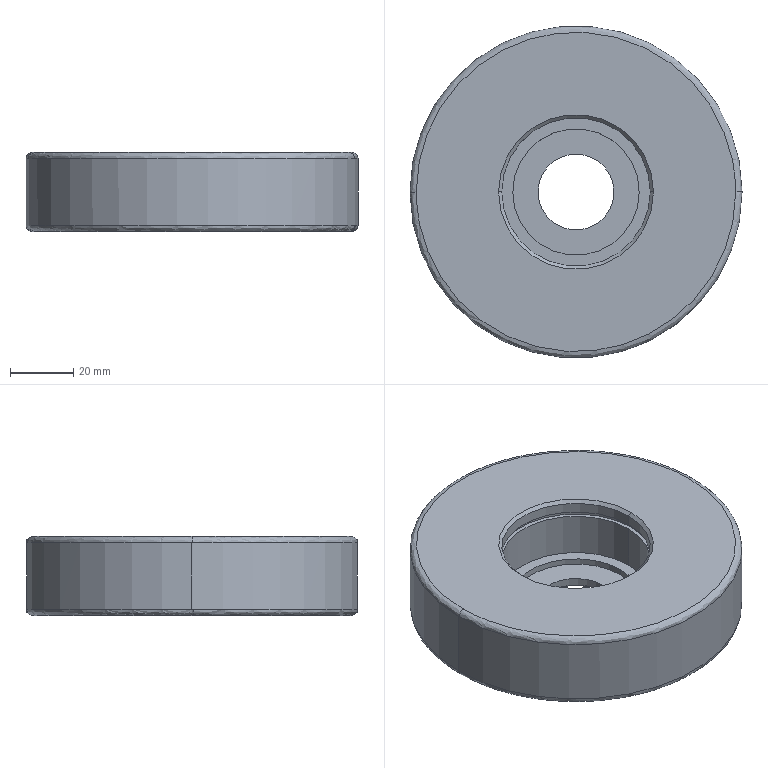Part | SolidWorks | features BaseBody 1 | 1 solid | 26 faces | box 105 x 105 x 25 mm | volume 176949 mm3 | cylinder 12 | plane 6 | spline 4 | cone 4 | commonest cylinder face diameters 47 x4 24 x2 40 x2 49.5 x2 105 x2
STEP:
#1=CARTESIAN_POINT('',(-52.5,0.,-23.));
#2=VERTEX_POINT('',#1);
#3=CARTESIAN_POINT('',(52.499,0.3289,-23.));
#4=VERTEX_POINT('',#3);
#5=CARTESIAN_POINT('',(0.,0.,-23.));
#6=DIRECTION('',(0.,0.,-1.));
#7=DIRECTION('',(-1.,-0.006265,0.));
#8=AXIS2_PLACEMENT_3D('',#5,#6,#7);
#9=CIRCLE('',#8,52.5);
#10=EDGE_CURVE('',#2,#4,#9,.T.);
#11=ORIENTED_EDGE('',*,*,#10,.T.);
#12=CARTESIAN_POINT('',(50.499,0.3164,-25.));
#13=VERTEX_POINT('',#12);
#14=CARTESIAN_POINT('',(50.499,0.3164,-23.));
#15=DIRECTION('',(-0.006265,1.,0.));
#16=DIRECTION('',(1.,0.006265,0.));
#17=AXIS2_PLACEMENT_3D('',#14,#15,#16);
#18=CIRCLE('',#17,2.);
#19=EDGE_CURVE('',#4,#13,#18,.T.);
#20=ORIENTED_EDGE('',*,*,#19,.T.);
#21=CARTESIAN_POINT('',(-50.5,0.,-25.));
#22=VERTEX_POINT('',#21);
#23=CARTESIAN_POINT('',(50.499,0.3164,-25.));
#24=CARTESIAN_POINT('',(49.87,100.685,-25.));
#25=CARTESIAN_POINT('',(-50.5,100.371,-25.));
#26=CARTESIAN_POINT('',(-50.5,0.,-25.));
#27=(BOUNDED_CURVE()B_SPLINE_CURVE(3,(#23,#24,#25,#26),.UNSPECIFIED.,.F.,.F.)B_SPLINE_CURVE_WITH_KNOTS((4,4),(0.001994,1.),.UNSPECIFIED.)CURVE()GEOMETRIC_REPRESENTATION_ITEM()RATIONAL_B_SPLINE_CURVE((1.,0.3354,0.3354,1.))REPRESENTATION_ITEM(''));
#28=EDGE_CURVE('',#13,#22,#27,.T.);
#29=ORIENTED_EDGE('',*,*,#28,.T.);
#30=CARTESIAN_POINT('',(-50.499,-0.3164,-25.));
#31=VERTEX_POINT('',#30);
#32=CARTESIAN_POINT('',(-50.5,0.,-25.));
#33=CARTESIAN_POINT('',(-50.5,-0.1055,-25.));
#34=CARTESIAN_POINT('',(-50.5,-0.2109,-25.));
#35=CARTESIAN_POINT('',(-50.499,-0.3164,-25.));
#36=(BOUNDED_CURVE()B_SPLINE_CURVE(3,(#32,#33,#34,#35),.UNSPECIFIED.,.F.,.F.)B_SPLINE_CURVE_WITH_KNOTS((4,4),(0.,0.001994),.UNSPECIFIED.)CURVE()GEOMETRIC_REPRESENTATION_ITEM()RATIONAL_B_SPLINE_CURVE((1.,1.,1.,1.))REPRESENTATION_ITEM(''));
#37=EDGE_CURVE('',#22,#31,#36,.T.);
#38=ORIENTED_EDGE('',*,*,#37,.T.);
#39=CARTESIAN_POINT('',(-52.499,-0.3289,-23.));
#40=VERTEX_POINT('',#39);
#41=CARTESIAN_POINT('',(-50.499,-0.3164,-23.));
#42=DIRECTION('',(0.006265,-1.,0.));
#43=DIRECTION('',(-1.,-0.006265,0.));
#44=AXIS2_PLACEMENT_3D('',#41,#42,#43);
#45=CIRCLE('',#44,2.);
#46=EDGE_CURVE('',#40,#31,#45,.T.);
#47=ORIENTED_EDGE('',*,*,#46,.F.);
#48=CARTESIAN_POINT('',(0.,0.,-23.));
#49=DIRECTION('',(0.,0.,-1.));
#50=DIRECTION('',(-1.,-0.006265,0.));
#51=AXIS2_PLACEMENT_3D('',#48,#49,#50);
#52=CIRCLE('',#51,52.5);
#53=EDGE_CURVE('',#40,#2,#52,.T.);
#54=ORIENTED_EDGE('',*,*,#53,.T.);
#55=EDGE_LOOP('',(#11,#20,#29,#38,#47,#54));
#56=FACE_OUTER_BOUND('',#55,.T.);
#57=CARTESIAN_POINT('',(52.499,0.3289,-23.));
#58=CARTESIAN_POINT('',(51.841,105.327,-23.));
#59=CARTESIAN_POINT('',(-53.157,104.669,-23.));
#60=CARTESIAN_POINT('',(-52.499,-0.3289,-23.));
#61=CARTESIAN_POINT('',(52.499,0.3289,-24.172));
#62=CARTESIAN_POINT('',(51.841,105.327,-24.172));
#63=CARTESIAN_POINT('',(-53.157,104.669,-24.172));
#64=CARTESIAN_POINT('',(-52.499,-0.3289,-24.172));
#65=CARTESIAN_POINT('',(51.671,0.3237,-25.));
#66=CARTESIAN_POINT('',(51.023,103.665,-25.));
#67=CARTESIAN_POINT('',(-52.318,103.017,-25.));
#68=CARTESIAN_POINT('',(-51.671,-0.3237,-25.));
#69=CARTESIAN_POINT('',(50.499,0.3164,-25.));
#70=CARTESIAN_POINT('',(49.866,101.314,-25.));
#71=CARTESIAN_POINT('',(-51.132,100.682,-25.));
#72=CARTESIAN_POINT('',(-50.499,-0.3164,-25.));
#73=(BOUNDED_SURFACE()B_SPLINE_SURFACE(3,3,((#57,#58,#59,#60),(#61,#62,#63,#64),(#65,#66,#67,#68),(#69,#70,#71,#72)),.UNSPECIFIED.,.F.,.F.,.T.)B_SPLINE_SURFACE_WITH_KNOTS((4,4),(4,4),(0.,1.),(0.,1.),.UNSPECIFIED.)GEOMETRIC_REPRESENTATION_ITEM()RATIONAL_B_SPLINE_SURFACE(((1.,0.3333,0.3333,1.),(0.8047,0.2682,0.2682,0.8047),(0.8047,0.2682,0.2682,0.8047),(1.,0.3333,0.3333,1.)))REPRESENTATION_ITEM('')SURFACE());
#74=ADVANCED_FACE('',(#56),#73,.T.);
#75=CARTESIAN_POINT('',(-50.5,0.,0.));
#76=VERTEX_POINT('',#75);
#77=CARTESIAN_POINT('',(50.5,0.2141,0.));
#78=VERTEX_POINT('',#77);
#79=CARTESIAN_POINT('',(-50.5,0.,0.));
#80=CARTESIAN_POINT('',(-50.5,100.573,0.));
#81=CARTESIAN_POINT('',(50.073,100.787,0.));
#82=CARTESIAN_POINT('',(50.5,0.2141,0.));
#83=(BOUNDED_CURVE()B_SPLINE_CURVE(3,(#79,#80,#81,#82),.UNSPECIFIED.,.F.,.F.)B_SPLINE_CURVE_WITH_KNOTS((4,4),(0.,0.9987),.UNSPECIFIED.)CURVE()GEOMETRIC_REPRESENTATION_ITEM()RATIONAL_B_SPLINE_CURVE((1.,0.3347,0.3347,1.))REPRESENTATION_ITEM(''));
#84=EDGE_CURVE('',#76,#78,#83,.T.);
#85=ORIENTED_EDGE('',*,*,#84,.T.);
#86=CARTESIAN_POINT('',(52.5,0.2226,-2.));
#87=VERTEX_POINT('',#86);
#88=CARTESIAN_POINT('',(50.5,0.2141,-2.));
#89=DIRECTION('',(-0.004241,1.,0.));
#90=DIRECTION('',(1.,0.004241,0.));
#91=AXIS2_PLACEMENT_3D('',#88,#89,#90);
#92=CIRCLE('',#91,2.);
#93=EDGE_CURVE('',#78,#87,#92,.T.);
#94=ORIENTED_EDGE('',*,*,#93,.T.);
#95=CARTESIAN_POINT('',(-52.5,0.,-2.));
#96=VERTEX_POINT('',#95);
#97=CARTESIAN_POINT('',(0.,0.,-2.));
#98=DIRECTION('',(0.,0.,-1.));
#99=DIRECTION('',(1.,0.,0.));
#100=AXIS2_PLACEMENT_3D('',#97,#98,#99);
#101=CIRCLE('',#100,52.5);
#102=EDGE_CURVE('',#96,#87,#101,.T.);
#103=ORIENTED_EDGE('',*,*,#102,.F.);
#104=CARTESIAN_POINT('',(-52.5,-0.2226,-2.));
#105=VERTEX_POINT('',#104);
#106=CARTESIAN_POINT('',(0.,0.,-2.));
#107=DIRECTION('',(0.,0.,-1.));
#108=DIRECTION('',(1.,0.,0.));
#109=AXIS2_PLACEMENT_3D('',#106,#107,#108);
#110=CIRCLE('',#109,52.5);
#111=EDGE_CURVE('',#105,#96,#110,.T.);
#112=ORIENTED_EDGE('',*,*,#111,.F.);
#113=CARTESIAN_POINT('',(-50.5,-0.2141,0.));
#114=VERTEX_POINT('',#113);
#115=CARTESIAN_POINT('',(-50.5,-0.2141,-2.));
#116=DIRECTION('',(0.004241,-1.,0.));
#117=DIRECTION('',(-1.,-0.004241,0.));
#118=AXIS2_PLACEMENT_3D('',#115,#116,#117);
#119=CIRCLE('',#118,2.);
#120=EDGE_CURVE('',#114,#105,#119,.T.);
#121=ORIENTED_EDGE('',*,*,#120,.F.);
#122=CARTESIAN_POINT('',(-50.5,-0.2141,0.));
#123=CARTESIAN_POINT('',(-50.5,-0.1428,0.));
#124=CARTESIAN_POINT('',(-50.5,-0.07138,0.));
#125=CARTESIAN_POINT('',(-50.5,0.,0.));
#126=(BOUNDED_CURVE()B_SPLINE_CURVE(3,(#122,#123,#124,#125),.UNSPECIFIED.,.F.,.F.)B_SPLINE_CURVE_WITH_KNOTS((4,4),(0.9987,1.),.UNSPECIFIED.)CURVE()GEOMETRIC_REPRESENTATION_ITEM()RATIONAL_B_SPLINE_CURVE((1.,1.,1.,1.))REPRESENTATION_ITEM(''));
#127=EDGE_CURVE('',#114,#76,#126,.T.);
#128=ORIENTED_EDGE('',*,*,#127,.T.);
#129=EDGE_LOOP('',(#85,#94,#103,#112,#121,#128));
#130=FACE_OUTER_BOUND('',#129,.T.);
#131=CARTESIAN_POINT('',(50.5,0.2141,0.));
#132=CARTESIAN_POINT('',(50.071,101.213,0.));
#133=CARTESIAN_POINT('',(-50.928,100.785,0.));
#134=CARTESIAN_POINT('',(-50.5,-0.2141,0.));
#135=CARTESIAN_POINT('',(51.671,0.2191,0.));
#136=CARTESIAN_POINT('',(51.233,103.561,0.));
#137=CARTESIAN_POINT('',(-52.109,103.123,0.));
#138=CARTESIAN_POINT('',(-51.671,-0.2191,0.));
#139=CARTESIAN_POINT('',(52.5,0.2226,-0.8284));
#140=CARTESIAN_POINT('',(52.054,105.222,-0.8284));
#141=CARTESIAN_POINT('',(-52.945,104.776,-0.8284));
#142=CARTESIAN_POINT('',(-52.5,-0.2226,-0.8284));
#143=CARTESIAN_POINT('',(52.5,0.2226,-2.));
#144=CARTESIAN_POINT('',(52.054,105.222,-2.));
#145=CARTESIAN_POINT('',(-52.945,104.776,-2.));
#146=CARTESIAN_POINT('',(-52.5,-0.2226,-2.));
#147=(BOUNDED_SURFACE()B_SPLINE_SURFACE(3,3,((#131,#132,#133,#134),(#135,#136,#137,#138),(#139,#140,#141,#142),(#143,#144,#145,#146)),.UNSPECIFIED.,.F.,.F.,.T.)B_SPLINE_SURFACE_WITH_KNOTS((4,4),(4,4),(0.,1.),(0.,1.),.UNSPECIFIED.)GEOMETRIC_REPRESENTATION_ITEM()RATIONAL_B_SPLINE_SURFACE(((1.,0.3333,0.3333,1.),(0.8047,0.2682,0.2682,0.8047),(0.8047,0.2682,0.2682,0.8047),(1.,0.3333,0.3333,1.)))REPRESENTATION_ITEM('')SURFACE());
#148=ADVANCED_FACE('',(#130),#147,.T.);
#149=CARTESIAN_POINT('',(12.,0.,-24.5));
#150=VERTEX_POINT('',#149);
#151=CARTESIAN_POINT('',(-12.,0.,-24.5));
#152=VERTEX_POINT('',#151);
#153=CARTESIAN_POINT('',(0.,0.,-24.5));
#154=DIRECTION('',(0.,0.,-1.));
#155=DIRECTION('',(0.,-1.,0.));
#156=AXIS2_PLACEMENT_3D('',#153,#154,#155);
#157=CIRCLE('',#156,12.);
#158=EDGE_CURVE('',#150,#152,#157,.T.);
#159=ORIENTED_EDGE('',*,*,#158,.F.);
#160=CARTESIAN_POINT('',(12.5,0.,-25.));
#161=VERTEX_POINT('',#160);
#162=CARTESIAN_POINT('',(12.5,0.,-25.));
#163=DIRECTION('',(0.7071,0.,-0.7071));
#164=VECTOR('',#163,1000.);
#165=LINE('',#162,#164);
#166=EDGE_CURVE('',#150,#161,#165,.T.);
#167=ORIENTED_EDGE('',*,*,#166,.T.);
#168=CARTESIAN_POINT('',(-12.5,0.,-25.));
#169=VERTEX_POINT('',#168);
#170=CARTESIAN_POINT('',(0.,0.,-25.));
#171=DIRECTION('',(0.,0.,-1.));
#172=DIRECTION('',(-1.,0.,0.));
#173=AXIS2_PLACEMENT_3D('',#170,#171,#172);
#174=CIRCLE('',#173,12.5);
#175=EDGE_CURVE('',#161,#169,#174,.T.);
#176=ORIENTED_EDGE('',*,*,#175,.T.);
#177=CARTESIAN_POINT('',(-12.5,0.,-25.));
#178=DIRECTION('',(-0.7071,0.,-0.7071));
#179=VECTOR('',#178,1000.);
#180=LINE('',#177,#179);
#181=EDGE_CURVE('',#152,#169,#180,.T.);
#182=ORIENTED_EDGE('',*,*,#181,.F.);
#183=EDGE_LOOP('',(#159,#167,#176,#182));
#184=FACE_OUTER_BOUND('',#183,.T.);
#185=CARTESIAN_POINT('',(0.,0.,-25.));
#186=DIRECTION('',(0.,0.,-1.));
#187=DIRECTION('',(-1.,0.,0.));
#188=AXIS2_PLACEMENT_3D('',#185,#186,#187);
#189=CONICAL_SURFACE('',#188,12.5,0.7854);
#190=ADVANCED_FACE('',(#184),#189,.F.);
#191=ORIENTED_EDGE('',*,*,#158,.T.);
#192=CARTESIAN_POINT('',(-12.,0.,-22.));
#193=VERTEX_POINT('',#192);
#194=CARTESIAN_POINT('',(-12.,0.,-26.25));
#195=DIRECTION('',(0.,0.,1.));
#196=VECTOR('',#195,1000.);
#197=LINE('',#194,#196);
#198=EDGE_CURVE('',#152,#193,#197,.T.);
#199=ORIENTED_EDGE('',*,*,#198,.T.);
#200=CARTESIAN_POINT('',(12.,0.,-22.));
#201=VERTEX_POINT('',#200);
#202=CARTESIAN_POINT('',(0.,0.,-22.));
#203=DIRECTION('',(0.,0.,-1.));
#204=DIRECTION('',(1.,0.,0.));
#205=AXIS2_PLACEMENT_3D('',#202,#203,#204);
#206=CIRCLE('',#205,12.);
#207=EDGE_CURVE('',#201,#193,#206,.T.);
#208=ORIENTED_EDGE('',*,*,#207,.F.);
#209=CARTESIAN_POINT('',(12.,0.,-26.25));
#210=DIRECTION('',(0.,0.,1.));
#211=VECTOR('',#210,1000.);
#212=LINE('',#209,#211);
#213=EDGE_CURVE('',#150,#201,#212,.T.);
#214=ORIENTED_EDGE('',*,*,#213,.F.);
#215=EDGE_LOOP('',(#191,#199,#208,#214));
#216=FACE_OUTER_BOUND('',#215,.T.);
#217=CARTESIAN_POINT('',(0.,0.,-26.25));
#218=DIRECTION('',(0.,0.,1.));
#219=DIRECTION('',(1.,0.,0.));
#220=AXIS2_PLACEMENT_3D('',#217,#218,#219);
#221=CYLINDRICAL_SURFACE('',#220,12.);
#222=ADVANCED_FACE('',(#216),#221,.F.);
#223=ORIENTED_EDGE('',*,*,#10,.F.);
#224=CARTESIAN_POINT('',(-52.5,0.,-26.25));
#225=DIRECTION('',(0.,0.,1.));
#226=VECTOR('',#225,1000.);
#227=LINE('',#224,#226);
#228=EDGE_CURVE('',#2,#96,#227,.T.);
#229=ORIENTED_EDGE('',*,*,#228,.T.);
#230=ORIENTED_EDGE('',*,*,#102,.T.);
#231=CARTESIAN_POINT('',(52.5,0.,-2.));
#232=VERTEX_POINT('',#231);
#233=CARTESIAN_POINT('',(0.,0.,-2.));
#234=DIRECTION('',(0.,0.,-1.));
#235=DIRECTION('',(1.,0.,0.));
#236=AXIS2_PLACEMENT_3D('',#233,#234,#235);
#237=CIRCLE('',#236,52.5);
#238=EDGE_CURVE('',#87,#232,#237,.T.);
#239=ORIENTED_EDGE('',*,*,#238,.T.);
#240=CARTESIAN_POINT('',(52.5,0.,-23.));
#241=VERTEX_POINT('',#240);
#242=CARTESIAN_POINT('',(52.5,0.,-26.25));
#243=DIRECTION('',(0.,0.,1.));
#244=VECTOR('',#243,1000.);
#245=LINE('',#242,#244);
#246=EDGE_CURVE('',#241,#232,#245,.T.);
#247=ORIENTED_EDGE('',*,*,#246,.F.);
#248=CARTESIAN_POINT('',(0.,0.,-23.));
#249=DIRECTION('',(0.,0.,-1.));
#250=DIRECTION('',(-1.,-0.006265,0.));
#251=AXIS2_PLACEMENT_3D('',#248,#249,#250);
#252=CIRCLE('',#251,52.5);
#253=EDGE_CURVE('',#4,#241,#252,.T.);
#254=ORIENTED_EDGE('',*,*,#253,.F.);
#255=EDGE_LOOP('',(#223,#229,#230,#239,#247,#254));
#256=FACE_OUTER_BOUND('',#255,.T.);
#257=CARTESIAN_POINT('',(0.,0.,-26.25));
#258=DIRECTION('',(0.,0.,1.));
#259=DIRECTION('',(1.,0.,0.));
#260=AXIS2_PLACEMENT_3D('',#257,#258,#259);
#261=CYLINDRICAL_SURFACE('',#260,52.5);
#262=ADVANCED_FACE('',(#256),#261,.T.);
#263=CARTESIAN_POINT('',(-20.,0.,-22.));
#264=VERTEX_POINT('',#263);
#265=CARTESIAN_POINT('',(20.,0.,-22.));
#266=VERTEX_POINT('',#265);
#267=CARTESIAN_POINT('',(0.,0.,-22.));
#268=DIRECTION('',(0.,0.,1.));
#269=DIRECTION('',(1.,0.,0.));
#270=AXIS2_PLACEMENT_3D('',#267,#268,#269);
#271=CIRCLE('',#270,20.);
#272=EDGE_CURVE('',#264,#266,#271,.T.);
#273=ORIENTED_EDGE('',*,*,#272,.F.);
#274=CARTESIAN_POINT('',(-20.,0.,-20.));
#275=VERTEX_POINT('',#274);
#276=CARTESIAN_POINT('',(-20.,0.,-26.25));
#277=DIRECTION('',(0.,0.,1.));
#278=VECTOR('',#277,1000.);
#279=LINE('',#276,#278);
#280=EDGE_CURVE('',#264,#275,#279,.T.);
#281=ORIENTED_EDGE('',*,*,#280,.T.);
#282=CARTESIAN_POINT('',(20.,0.,-20.));
#283=VERTEX_POINT('',#282);
#284=CARTESIAN_POINT('',(0.,0.,-20.));
#285=DIRECTION('',(0.,0.,-1.));
#286=DIRECTION('',(1.,0.,0.));
#287=AXIS2_PLACEMENT_3D('',#284,#285,#286);
#288=CIRCLE('',#287,20.);
#289=EDGE_CURVE('',#283,#275,#288,.T.);
#290=ORIENTED_EDGE('',*,*,#289,.F.);
#291=CARTESIAN_POINT('',(20.,0.,-26.25));
#292=DIRECTION('',(0.,0.,1.));
#293=VECTOR('',#292,1000.);
#294=LINE('',#291,#293);
#295=EDGE_CURVE('',#266,#283,#294,.T.);
#296=ORIENTED_EDGE('',*,*,#295,.F.);
#297=EDGE_LOOP('',(#273,#281,#290,#296));
#298=FACE_OUTER_BOUND('',#297,.T.);
#299=CARTESIAN_POINT('',(0.,0.,-26.25));
#300=DIRECTION('',(0.,0.,1.));
#301=DIRECTION('',(1.,0.,0.));
#302=AXIS2_PLACEMENT_3D('',#299,#300,#301);
#303=CYLINDRICAL_SURFACE('',#302,20.);
#304=ADVANCED_FACE('',(#298),#303,.F.);
#305=CARTESIAN_POINT('',(-23.5,0.,-1.));
#306=VERTEX_POINT('',#305);
#307=CARTESIAN_POINT('',(23.5,0.,-1.));
#308=VERTEX_POINT('',#307);
#309=CARTESIAN_POINT('',(0.,0.,-1.));
#310=DIRECTION('',(0.,0.,1.));
#311=DIRECTION('',(0.,-1.,0.));
#312=AXIS2_PLACEMENT_3D('',#309,#310,#311);
#313=CIRCLE('',#312,23.5);
#314=EDGE_CURVE('',#306,#308,#313,.T.);
#315=ORIENTED_EDGE('',*,*,#314,.F.);
#316=CARTESIAN_POINT('',(-24.5,0.,0.));
#317=VERTEX_POINT('',#316);
#318=CARTESIAN_POINT('',(-24.5,0.,0.));
#319=DIRECTION('',(-0.7071,0.,0.7071));
#320=VECTOR('',#319,1000.);
#321=LINE('',#318,#320);
#322=EDGE_CURVE('',#306,#317,#321,.T.);
#323=ORIENTED_EDGE('',*,*,#322,.T.);
#324=CARTESIAN_POINT('',(24.5,0.,0.));
#325=VERTEX_POINT('',#324);
#326=CARTESIAN_POINT('',(0.,0.,0.));
#327=DIRECTION('',(0.,0.,-1.));
#328=DIRECTION('',(1.,0.,0.));
#329=AXIS2_PLACEMENT_3D('',#326,#327,#328);
#330=CIRCLE('',#329,24.5);
#331=EDGE_CURVE('',#325,#317,#330,.T.);
#332=ORIENTED_EDGE('',*,*,#331,.F.);
#333=CARTESIAN_POINT('',(24.5,0.,0.));
#334=DIRECTION('',(0.7071,0.,0.7071));
#335=VECTOR('',#334,1000.);
#336=LINE('',#333,#335);
#337=EDGE_CURVE('',#308,#325,#336,.T.);
#338=ORIENTED_EDGE('',*,*,#337,.F.);
#339=EDGE_LOOP('',(#315,#323,#332,#338));
#340=FACE_OUTER_BOUND('',#339,.T.);
#341=CARTESIAN_POINT('',(0.,0.,0.));
#342=DIRECTION('',(0.,0.,1.));
#343=DIRECTION('',(1.,0.,0.));
#344=AXIS2_PLACEMENT_3D('',#341,#342,#343);
#345=CONICAL_SURFACE('',#344,24.5,0.7854);
#346=ADVANCED_FACE('',(#340),#345,.F.);
#347=CARTESIAN_POINT('',(-23.5,0.,-20.));
#348=VERTEX_POINT('',#347);
#349=CARTESIAN_POINT('',(23.5,0.,-20.));
#350=VERTEX_POINT('',#349);
#351=CARTESIAN_POINT('',(0.,0.,-20.));
#352=DIRECTION('',(0.,0.,1.));
#353=DIRECTION('',(1.,0.,0.));
#354=AXIS2_PLACEMENT_3D('',#351,#352,#353);
#355=CIRCLE('',#354,23.5);
#356=EDGE_CURVE('',#348,#350,#355,.T.);
#357=ORIENTED_EDGE('',*,*,#356,.F.);
#358=CARTESIAN_POINT('',(-23.5,0.,-6.));
#359=VERTEX_POINT('',#358);
#360=CARTESIAN_POINT('',(-23.5,0.,-26.25));
#361=DIRECTION('',(0.,0.,1.));
#362=VECTOR('',#361,1000.);
#363=LINE('',#360,#362);
#364=EDGE_CURVE('',#348,#359,#363,.T.);
#365=ORIENTED_EDGE('',*,*,#364,.T.);
#366=CARTESIAN_POINT('',(23.5,0.,-6.));
#367=VERTEX_POINT('',#366);
#368=CARTESIAN_POINT('',(0.,0.,-6.));
#369=DIRECTION('',(0.,0.,-1.));
#370=DIRECTION('',(1.,0.,0.));
#371=AXIS2_PLACEMENT_3D('',#368,#369,#370);
#372=CIRCLE('',#371,23.5);
#373=EDGE_CURVE('',#367,#359,#372,.T.);
#374=ORIENTED_EDGE('',*,*,#373,.F.);
#375=CARTESIAN_POINT('',(23.5,0.,-26.25));
#376=DIRECTION('',(0.,0.,1.));
#377=VECTOR('',#376,1000.);
#378=LINE('',#375,#377);
#379=EDGE_CURVE('',#350,#367,#378,.T.);
#380=ORIENTED_EDGE('',*,*,#379,.F.);
#381=EDGE_LOOP('',(#357,#365,#374,#380));
#382=FACE_OUTER_BOUND('',#381,.T.);
#383=CARTESIAN_POINT('',(0.,0.,-26.25));
#384=DIRECTION('',(0.,0.,1.));
#385=DIRECTION('',(1.,0.,0.));
#386=AXIS2_PLACEMENT_3D('',#383,#384,#385);
#387=CYLINDRICAL_SURFACE('',#386,23.5);
#388=ADVANCED_FACE('',(#382),#387,.F.);
#389=CARTESIAN_POINT('',(-23.5,0.,-4.3));
#390=VERTEX_POINT('',#389);
#391=CARTESIAN_POINT('',(23.5,0.,-4.3));
#392=VERTEX_POINT('',#391);
#393=CARTESIAN_POINT('',(0.,0.,-4.3));
#394=DIRECTION('',(0.,0.,1.));
#395=DIRECTION('',(1.,0.,0.));
#396=AXIS2_PLACEMENT_3D('',#393,#394,#395);
#397=CIRCLE('',#396,23.5);
#398=EDGE_CURVE('',#390,#392,#397,.T.);
#399=ORIENTED_EDGE('',*,*,#398,.F.);
#400=CARTESIAN_POINT('',(-23.5,0.,-26.25));
#401=DIRECTION('',(0.,0.,1.));
#402=VECTOR('',#401,1000.);
#403=LINE('',#400,#402);
#404=EDGE_CURVE('',#390,#306,#403,.T.);
#405=ORIENTED_EDGE('',*,*,#404,.T.);
#406=ORIENTED_EDGE('',*,*,#314,.T.);
#407=CARTESIAN_POINT('',(23.5,0.,-26.25));
#408=DIRECTION('',(0.,0.,1.));
#409=VECTOR('',#408,1000.);
#410=LINE('',#407,#409);
#411=EDGE_CURVE('',#392,#308,#410,.T.);
#412=ORIENTED_EDGE('',*,*,#411,.F.);
#413=EDGE_LOOP('',(#399,#405,#406,#412));
#414=FACE_OUTER_BOUND('',#413,.T.);
#415=CARTESIAN_POINT('',(0.,0.,-26.25));
#416=DIRECTION('',(0.,0.,1.));
#417=DIRECTION('',(1.,0.,0.));
#418=AXIS2_PLACEMENT_3D('',#415,#416,#417);
#419=CYLINDRICAL_SURFACE('',#418,23.5);
#420=ADVANCED_FACE('',(#414),#419,.F.);
#421=CARTESIAN_POINT('',(-24.75,0.,-6.));
#422=VERTEX_POINT('',#421);
#423=CARTESIAN_POINT('',(24.75,0.,-6.));
#424=VERTEX_POINT('',#423);
#425=CARTESIAN_POINT('',(0.,0.,-6.));
#426=DIRECTION('',(0.,0.,1.));
#427=DIRECTION('',(1.,0.,0.));
#428=AXIS2_PLACEMENT_3D('',#425,#426,#427);
#429=CIRCLE('',#428,24.75);
#430=EDGE_CURVE('',#422,#424,#429,.T.);
#431=ORIENTED_EDGE('',*,*,#430,.F.);
#432=CARTESIAN_POINT('',(-24.75,0.,-4.3));
#433=VERTEX_POINT('',#432);
#434=CARTESIAN_POINT('',(-24.75,0.,-26.25));
#435=DIRECTION('',(0.,0.,1.));
#436=VECTOR('',#435,1000.);
#437=LINE('',#434,#436);
#438=EDGE_CURVE('',#422,#433,#437,.T.);
#439=ORIENTED_EDGE('',*,*,#438,.T.);
#440=CARTESIAN_POINT('',(24.75,0.,-4.3));
#441=VERTEX_POINT('',#440);
#442=CARTESIAN_POINT('',(0.,0.,-4.3));
#443=DIRECTION('',(0.,0.,1.));
#444=DIRECTION('',(1.,0.,0.));
#445=AXIS2_PLACEMENT_3D('',#442,#443,#444);
#446=CIRCLE('',#445,24.75);
#447=EDGE_CURVE('',#433,#441,#446,.T.);
#448=ORIENTED_EDGE('',*,*,#447,.T.);
#449=CARTESIAN_POINT('',(24.75,0.,-26.25));
#450=DIRECTION('',(0.,0.,1.));
#451=VECTOR('',#450,1000.);
#452=LINE('',#449,#451);
#453=EDGE_CURVE('',#424,#441,#452,.T.);
#454=ORIENTED_EDGE('',*,*,#453,.F.);
#455=EDGE_LOOP('',(#431,#439,#448,#454));
#456=FACE_OUTER_BOUND('',#455,.T.);
#457=CARTESIAN_POINT('',(0.,0.,-26.25));
#458=DIRECTION('',(0.,0.,1.));
#459=DIRECTION('',(1.,0.,0.));
#460=AXIS2_PLACEMENT_3D('',#457,#458,#459);
#461=CYLINDRICAL_SURFACE('',#460,24.75);
#462=ADVANCED_FACE('',(#456),#461,.F.);
#463=CARTESIAN_POINT('',(0.,0.,-25.));
#464=DIRECTION('',(0.,0.,-1.));
#465=DIRECTION('',(-1.,0.,0.));
#466=AXIS2_PLACEMENT_3D('',#463,#464,#465);
#467=CIRCLE('',#466,12.5);
#468=EDGE_CURVE('',#169,#161,#467,.T.);
#469=ORIENTED_EDGE('',*,*,#468,.F.);
#470=ORIENTED_EDGE('',*,*,#175,.F.);
#471=EDGE_LOOP('',(#469,#470));
#472=FACE_BOUND('',#471,.T.);
#473=ORIENTED_EDGE('',*,*,#37,.F.);
#474=ORIENTED_EDGE('',*,*,#28,.F.);
#475=CARTESIAN_POINT('',(50.5,0.,-25.));
#476=VERTEX_POINT('',#475);
#477=CARTESIAN_POINT('',(50.5,0.,-25.));
#478=CARTESIAN_POINT('',(50.5,0.1055,-25.));
#479=CARTESIAN_POINT('',(50.5,0.2109,-25.));
#480=CARTESIAN_POINT('',(50.499,0.3164,-25.));
#481=(BOUNDED_CURVE()B_SPLINE_CURVE(3,(#477,#478,#479,#480),.UNSPECIFIED.,.F.,.T.)B_SPLINE_CURVE_WITH_KNOTS((4,4),(0.,0.001994),.UNSPECIFIED.)CURVE()GEOMETRIC_REPRESENTATION_ITEM()RATIONAL_B_SPLINE_CURVE((1.,1.,1.,1.))REPRESENTATION_ITEM(''));
#482=EDGE_CURVE('',#476,#13,#481,.T.);
#483=ORIENTED_EDGE('',*,*,#482,.F.);
#484=CARTESIAN_POINT('',(-50.499,-0.3164,-25.));
#485=CARTESIAN_POINT('',(-49.87,-100.685,-25.));
#486=CARTESIAN_POINT('',(50.5,-100.371,-25.));
#487=CARTESIAN_POINT('',(50.5,0.,-25.));
#488=(BOUNDED_CURVE()B_SPLINE_CURVE(3,(#484,#485,#486,#487),.UNSPECIFIED.,.F.,.F.)B_SPLINE_CURVE_WITH_KNOTS((4,4),(0.001994,1.),.UNSPECIFIED.)CURVE()GEOMETRIC_REPRESENTATION_ITEM()RATIONAL_B_SPLINE_CURVE((1.,0.3354,0.3354,1.))REPRESENTATION_ITEM(''));
#489=EDGE_CURVE('',#31,#476,#488,.T.);
#490=ORIENTED_EDGE('',*,*,#489,.F.);
#491=EDGE_LOOP('',(#473,#474,#483,#490));
#492=FACE_OUTER_BOUND('',#491,.T.);
#493=CARTESIAN_POINT('',(0.,0.,-25.));
#494=DIRECTION('',(0.,0.,1.));
#495=DIRECTION('',(1.,0.,0.));
#496=AXIS2_PLACEMENT_3D('',#493,#494,#495);
#497=PLANE('',#496);
#498=ADVANCED_FACE('',(#472,#492),#497,.F.);
#499=ORIENTED_EDGE('',*,*,#166,.F.);
#500=CARTESIAN_POINT('',(0.,0.,-24.5));
#501=DIRECTION('',(0.,0.,-1.));
#502=DIRECTION('',(0.,-1.,0.));
#503=AXIS2_PLACEMENT_3D('',#500,#501,#502);
#504=CIRCLE('',#503,12.);
#505=EDGE_CURVE('',#152,#150,#504,.T.);
#506=ORIENTED_EDGE('',*,*,#505,.F.);
#507=ORIENTED_EDGE('',*,*,#181,.T.);
#508=ORIENTED_EDGE('',*,*,#468,.T.);
#509=EDGE_LOOP('',(#499,#506,#507,#508));
#510=FACE_OUTER_BOUND('',#509,.T.);
#511=CARTESIAN_POINT('',(0.,0.,-25.));
#512=DIRECTION('',(0.,0.,-1.));
#513=DIRECTION('',(-1.,0.,0.));
#514=AXIS2_PLACEMENT_3D('',#511,#512,#513);
#515=CONICAL_SURFACE('',#514,12.5,0.7854);
#516=ADVANCED_FACE('',(#510),#515,.F.);
#517=ORIENTED_EDGE('',*,*,#19,.F.);
#518=ORIENTED_EDGE('',*,*,#253,.T.);
#519=CARTESIAN_POINT('',(0.,0.,-23.));
#520=DIRECTION('',(0.,0.,-1.));
#521=DIRECTION('',(-1.,-0.006265,0.));
#522=AXIS2_PLACEMENT_3D('',#519,#520,#521);
#523=CIRCLE('',#522,52.5);
#524=EDGE_CURVE('',#241,#40,#523,.T.);
#525=ORIENTED_EDGE('',*,*,#524,.T.);
#526=ORIENTED_EDGE('',*,*,#46,.T.);
#527=ORIENTED_EDGE('',*,*,#489,.T.);
#528=ORIENTED_EDGE('',*,*,#482,.T.);
#529=EDGE_LOOP('',(#517,#518,#525,#526,#527,#528));
#530=FACE_OUTER_BOUND('',#529,.T.);
#531=CARTESIAN_POINT('',(-52.499,-0.3289,-23.));
#532=CARTESIAN_POINT('',(-51.841,-105.327,-23.));
#533=CARTESIAN_POINT('',(53.157,-104.669,-23.));
#534=CARTESIAN_POINT('',(52.499,0.3289,-23.));
#535=CARTESIAN_POINT('',(-52.499,-0.3289,-24.172));
#536=CARTESIAN_POINT('',(-51.841,-105.327,-24.172));
#537=CARTESIAN_POINT('',(53.157,-104.669,-24.172));
#538=CARTESIAN_POINT('',(52.499,0.3289,-24.172));
#539=CARTESIAN_POINT('',(-51.671,-0.3237,-25.));
#540=CARTESIAN_POINT('',(-51.023,-103.665,-25.));
#541=CARTESIAN_POINT('',(52.318,-103.017,-25.));
#542=CARTESIAN_POINT('',(51.671,0.3237,-25.));
#543=CARTESIAN_POINT('',(-50.499,-0.3164,-25.));
#544=CARTESIAN_POINT('',(-49.866,-101.314,-25.));
#545=CARTESIAN_POINT('',(51.132,-100.682,-25.));
#546=CARTESIAN_POINT('',(50.499,0.3164,-25.));
#547=(BOUNDED_SURFACE()B_SPLINE_SURFACE(3,3,((#531,#532,#533,#534),(#535,#536,#537,#538),(#539,#540,#541,#542),(#543,#544,#545,#546)),.UNSPECIFIED.,.F.,.F.,.T.)B_SPLINE_SURFACE_WITH_KNOTS((4,4),(4,4),(0.,1.),(0.,1.),.UNSPECIFIED.)GEOMETRIC_REPRESENTATION_ITEM()RATIONAL_B_SPLINE_SURFACE(((1.,0.3333,0.3333,1.),(0.8047,0.2682,0.2682,0.8047),(0.8047,0.2682,0.2682,0.8047),(1.,0.3333,0.3333,1.)))REPRESENTATION_ITEM('')SURFACE());
#548=ADVANCED_FACE('',(#530),#547,.T.);
#549=ORIENTED_EDGE('',*,*,#198,.F.);
#550=ORIENTED_EDGE('',*,*,#505,.T.);
#551=ORIENTED_EDGE('',*,*,#213,.T.);
#552=CARTESIAN_POINT('',(0.,0.,-22.));
#553=DIRECTION('',(0.,0.,-1.));
#554=DIRECTION('',(1.,0.,0.));
#555=AXIS2_PLACEMENT_3D('',#552,#553,#554);
#556=CIRCLE('',#555,12.);
#557=EDGE_CURVE('',#193,#201,#556,.T.);
#558=ORIENTED_EDGE('',*,*,#557,.F.);
#559=EDGE_LOOP('',(#549,#550,#551,#558));
#560=FACE_OUTER_BOUND('',#559,.T.);
#561=CARTESIAN_POINT('',(0.,0.,-26.25));
#562=DIRECTION('',(0.,0.,1.));
#563=DIRECTION('',(1.,0.,0.));
#564=AXIS2_PLACEMENT_3D('',#561,#562,#563);
#565=CYLINDRICAL_SURFACE('',#564,12.);
#566=ADVANCED_FACE('',(#560),#565,.F.);
#567=ORIENTED_EDGE('',*,*,#228,.F.);
#568=ORIENTED_EDGE('',*,*,#53,.F.);
#569=ORIENTED_EDGE('',*,*,#524,.F.);
#570=ORIENTED_EDGE('',*,*,#246,.T.);
#571=CARTESIAN_POINT('',(0.,0.,-2.));
#572=DIRECTION('',(0.,0.,-1.));
#573=DIRECTION('',(1.,0.,0.));
#574=AXIS2_PLACEMENT_3D('',#571,#572,#573);
#575=CIRCLE('',#574,52.5);
#576=EDGE_CURVE('',#232,#105,#575,.T.);
#577=ORIENTED_EDGE('',*,*,#576,.T.);
#578=ORIENTED_EDGE('',*,*,#111,.T.);
#579=EDGE_LOOP('',(#567,#568,#569,#570,#577,#578));
#580=FACE_OUTER_BOUND('',#579,.T.);
#581=CARTESIAN_POINT('',(0.,0.,-26.25));
#582=DIRECTION('',(0.,0.,1.));
#583=DIRECTION('',(1.,0.,0.));
#584=AXIS2_PLACEMENT_3D('',#581,#582,#583);
#585=CYLINDRICAL_SURFACE('',#584,52.5);
#586=ADVANCED_FACE('',(#580),#585,.T.);
#587=ORIENTED_EDGE('',*,*,#207,.T.);
#588=ORIENTED_EDGE('',*,*,#557,.T.);
#589=EDGE_LOOP('',(#587,#588));
#590=FACE_BOUND('',#589,.T.);
#591=CARTESIAN_POINT('',(0.,0.,-22.));
#592=DIRECTION('',(0.,0.,1.));
#593=DIRECTION('',(1.,0.,0.));
#594=AXIS2_PLACEMENT_3D('',#591,#592,#593);
#595=CIRCLE('',#594,20.);
#596=EDGE_CURVE('',#266,#264,#595,.T.);
#597=ORIENTED_EDGE('',*,*,#596,.T.);
#598=ORIENTED_EDGE('',*,*,#272,.T.);
#599=EDGE_LOOP('',(#597,#598));
#600=FACE_OUTER_BOUND('',#599,.T.);
#601=CARTESIAN_POINT('',(0.,0.,-22.));
#602=DIRECTION('',(0.,0.,1.));
#603=DIRECTION('',(1.,0.,0.));
#604=AXIS2_PLACEMENT_3D('',#601,#602,#603);
#605=PLANE('',#604);
#606=ADVANCED_FACE('',(#590,#600),#605,.T.);
#607=ORIENTED_EDGE('',*,*,#93,.F.);
#608=CARTESIAN_POINT('',(50.5,0.,0.));
#609=VERTEX_POINT('',#608);
#610=CARTESIAN_POINT('',(50.5,0.2141,0.));
#611=CARTESIAN_POINT('',(50.5,0.1428,0.));
#612=CARTESIAN_POINT('',(50.5,0.07138,0.));
#613=CARTESIAN_POINT('',(50.5,0.,0.));
#614=(BOUNDED_CURVE()B_SPLINE_CURVE(3,(#610,#611,#612,#613),.UNSPECIFIED.,.F.,.F.)B_SPLINE_CURVE_WITH_KNOTS((4,4),(0.9987,1.),.UNSPECIFIED.)CURVE()GEOMETRIC_REPRESENTATION_ITEM()RATIONAL_B_SPLINE_CURVE((1.,1.,1.,1.))REPRESENTATION_ITEM(''));
#615=EDGE_CURVE('',#78,#609,#614,.T.);
#616=ORIENTED_EDGE('',*,*,#615,.T.);
#617=CARTESIAN_POINT('',(50.5,0.,0.));
#618=CARTESIAN_POINT('',(50.5,-100.573,0.));
#619=CARTESIAN_POINT('',(-50.073,-100.787,0.));
#620=CARTESIAN_POINT('',(-50.5,-0.2141,0.));
#621=(BOUNDED_CURVE()B_SPLINE_CURVE(3,(#617,#618,#619,#620),.UNSPECIFIED.,.F.,.F.)B_SPLINE_CURVE_WITH_KNOTS((4,4),(0.,0.9987),.UNSPECIFIED.)CURVE()GEOMETRIC_REPRESENTATION_ITEM()RATIONAL_B_SPLINE_CURVE((1.,0.3347,0.3347,1.))REPRESENTATION_ITEM(''));
#622=EDGE_CURVE('',#609,#114,#621,.T.);
#623=ORIENTED_EDGE('',*,*,#622,.T.);
#624=ORIENTED_EDGE('',*,*,#120,.T.);
#625=ORIENTED_EDGE('',*,*,#576,.F.);
#626=ORIENTED_EDGE('',*,*,#238,.F.);
#627=EDGE_LOOP('',(#607,#616,#623,#624,#625,#626));
#628=FACE_OUTER_BOUND('',#627,.T.);
#629=CARTESIAN_POINT('',(-50.5,-0.2141,0.));
#630=CARTESIAN_POINT('',(-50.071,-101.213,0.));
#631=CARTESIAN_POINT('',(50.928,-100.785,0.));
#632=CARTESIAN_POINT('',(50.5,0.2141,0.));
#633=CARTESIAN_POINT('',(-51.671,-0.2191,0.));
#634=CARTESIAN_POINT('',(-51.233,-103.561,0.));
#635=CARTESIAN_POINT('',(52.109,-103.123,0.));
#636=CARTESIAN_POINT('',(51.671,0.2191,0.));
#637=CARTESIAN_POINT('',(-52.5,-0.2226,-0.8284));
#638=CARTESIAN_POINT('',(-52.054,-105.222,-0.8284));
#639=CARTESIAN_POINT('',(52.945,-104.776,-0.8284));
#640=CARTESIAN_POINT('',(52.5,0.2226,-0.8284));
#641=CARTESIAN_POINT('',(-52.5,-0.2226,-2.));
#642=CARTESIAN_POINT('',(-52.054,-105.222,-2.));
#643=CARTESIAN_POINT('',(52.945,-104.776,-2.));
#644=CARTESIAN_POINT('',(52.5,0.2226,-2.));
#645=(BOUNDED_SURFACE()B_SPLINE_SURFACE(3,3,((#629,#630,#631,#632),(#633,#634,#635,#636),(#637,#638,#639,#640),(#641,#642,#643,#644)),.UNSPECIFIED.,.F.,.F.,.F.)B_SPLINE_SURFACE_WITH_KNOTS((4,4),(4,4),(0.,1.),(0.,1.),.UNSPECIFIED.)GEOMETRIC_REPRESENTATION_ITEM()RATIONAL_B_SPLINE_SURFACE(((1.,0.3333,0.3333,1.),(0.8047,0.2682,0.2682,0.8047),(0.8047,0.2682,0.2682,0.8047),(1.,0.3333,0.3333,1.)))REPRESENTATION_ITEM('')SURFACE());
#646=ADVANCED_FACE('',(#628),#645,.T.);
#647=ORIENTED_EDGE('',*,*,#280,.F.);
#648=ORIENTED_EDGE('',*,*,#596,.F.);
#649=ORIENTED_EDGE('',*,*,#295,.T.);
#650=CARTESIAN_POINT('',(0.,0.,-20.));
#651=DIRECTION('',(0.,0.,-1.));
#652=DIRECTION('',(1.,0.,0.));
#653=AXIS2_PLACEMENT_3D('',#650,#651,#652);
#654=CIRCLE('',#653,20.);
#655=EDGE_CURVE('',#275,#283,#654,.T.);
#656=ORIENTED_EDGE('',*,*,#655,.F.);
#657=EDGE_LOOP('',(#647,#648,#649,#656));
#658=FACE_OUTER_BOUND('',#657,.T.);
#659=CARTESIAN_POINT('',(0.,0.,-26.25));
#660=DIRECTION('',(0.,0.,1.));
#661=DIRECTION('',(1.,0.,0.));
#662=AXIS2_PLACEMENT_3D('',#659,#660,#661);
#663=CYLINDRICAL_SURFACE('',#662,20.);
#664=ADVANCED_FACE('',(#658),#663,.F.);
#665=ORIENTED_EDGE('',*,*,#331,.T.);
#666=CARTESIAN_POINT('',(0.,0.,0.));
#667=DIRECTION('',(0.,0.,-1.));
#668=DIRECTION('',(1.,0.,0.));
#669=AXIS2_PLACEMENT_3D('',#666,#667,#668);
#670=CIRCLE('',#669,24.5);
#671=EDGE_CURVE('',#317,#325,#670,.T.);
#672=ORIENTED_EDGE('',*,*,#671,.T.);
#673=EDGE_LOOP('',(#665,#672));
#674=FACE_BOUND('',#673,.T.);
#675=ORIENTED_EDGE('',*,*,#84,.F.);
#676=ORIENTED_EDGE('',*,*,#127,.F.);
#677=ORIENTED_EDGE('',*,*,#622,.F.);
#678=ORIENTED_EDGE('',*,*,#615,.F.);
#679=EDGE_LOOP('',(#675,#676,#677,#678));
#680=FACE_OUTER_BOUND('',#679,.T.);
#681=CARTESIAN_POINT('',(0.,0.,0.));
#682=DIRECTION('',(0.,0.,1.));
#683=DIRECTION('',(1.,0.,0.));
#684=AXIS2_PLACEMENT_3D('',#681,#682,#683);
#685=PLANE('',#684);
#686=ADVANCED_FACE('',(#674,#680),#685,.T.);
#687=ORIENTED_EDGE('',*,*,#289,.T.);
#688=ORIENTED_EDGE('',*,*,#655,.T.);
#689=EDGE_LOOP('',(#687,#688));
#690=FACE_BOUND('',#689,.T.);
#691=CARTESIAN_POINT('',(0.,0.,-20.));
#692=DIRECTION('',(0.,0.,1.));
#693=DIRECTION('',(1.,0.,0.));
#694=AXIS2_PLACEMENT_3D('',#691,#692,#693);
#695=CIRCLE('',#694,23.5);
#696=EDGE_CURVE('',#350,#348,#695,.T.);
#697=ORIENTED_EDGE('',*,*,#696,.T.);
#698=ORIENTED_EDGE('',*,*,#356,.T.);
#699=EDGE_LOOP('',(#697,#698));
#700=FACE_OUTER_BOUND('',#699,.T.);
#701=CARTESIAN_POINT('',(0.,0.,-20.));
#702=DIRECTION('',(0.,0.,1.));
#703=DIRECTION('',(1.,0.,0.));
#704=AXIS2_PLACEMENT_3D('',#701,#702,#703);
#705=PLANE('',#704);
#706=ADVANCED_FACE('',(#690,#700),#705,.T.);
#707=ORIENTED_EDGE('',*,*,#322,.F.);
#708=CARTESIAN_POINT('',(0.,0.,-1.));
#709=DIRECTION('',(0.,0.,1.));
#710=DIRECTION('',(0.,-1.,0.));
#711=AXIS2_PLACEMENT_3D('',#708,#709,#710);
#712=CIRCLE('',#711,23.5);
#713=EDGE_CURVE('',#308,#306,#712,.T.);
#714=ORIENTED_EDGE('',*,*,#713,.F.);
#715=ORIENTED_EDGE('',*,*,#337,.T.);
#716=ORIENTED_EDGE('',*,*,#671,.F.);
#717=EDGE_LOOP('',(#707,#714,#715,#716));
#718=FACE_OUTER_BOUND('',#717,.T.);
#719=CARTESIAN_POINT('',(0.,0.,0.));
#720=DIRECTION('',(0.,0.,1.));
#721=DIRECTION('',(1.,0.,0.));
#722=AXIS2_PLACEMENT_3D('',#719,#720,#721);
#723=CONICAL_SURFACE('',#722,24.5,0.7854);
#724=ADVANCED_FACE('',(#718),#723,.F.);
#725=ORIENTED_EDGE('',*,*,#364,.F.);
#726=ORIENTED_EDGE('',*,*,#696,.F.);
#727=ORIENTED_EDGE('',*,*,#379,.T.);
#728=CARTESIAN_POINT('',(0.,0.,-6.));
#729=DIRECTION('',(0.,0.,-1.));
#730=DIRECTION('',(1.,0.,0.));
#731=AXIS2_PLACEMENT_3D('',#728,#729,#730);
#732=CIRCLE('',#731,23.5);
#733=EDGE_CURVE('',#359,#367,#732,.T.);
#734=ORIENTED_EDGE('',*,*,#733,.F.);
#735=EDGE_LOOP('',(#725,#726,#727,#734));
#736=FACE_OUTER_BOUND('',#735,.T.);
#737=CARTESIAN_POINT('',(0.,0.,-26.25));
#738=DIRECTION('',(0.,0.,1.));
#739=DIRECTION('',(1.,0.,0.));
#740=AXIS2_PLACEMENT_3D('',#737,#738,#739);
#741=CYLINDRICAL_SURFACE('',#740,23.5);
#742=ADVANCED_FACE('',(#736),#741,.F.);
#743=ORIENTED_EDGE('',*,*,#404,.F.);
#744=CARTESIAN_POINT('',(0.,0.,-4.3));
#745=DIRECTION('',(0.,0.,1.));
#746=DIRECTION('',(1.,0.,0.));
#747=AXIS2_PLACEMENT_3D('',#744,#745,#746);
#748=CIRCLE('',#747,23.5);
#749=EDGE_CURVE('',#392,#390,#748,.T.);
#750=ORIENTED_EDGE('',*,*,#749,.F.);
#751=ORIENTED_EDGE('',*,*,#411,.T.);
#752=ORIENTED_EDGE('',*,*,#713,.T.);
#753=EDGE_LOOP('',(#743,#750,#751,#752));
#754=FACE_OUTER_BOUND('',#753,.T.);
#755=CARTESIAN_POINT('',(0.,0.,-26.25));
#756=DIRECTION('',(0.,0.,1.));
#757=DIRECTION('',(1.,0.,0.));
#758=AXIS2_PLACEMENT_3D('',#755,#756,#757);
#759=CYLINDRICAL_SURFACE('',#758,23.5);
#760=ADVANCED_FACE('',(#754),#759,.F.);
#761=ORIENTED_EDGE('',*,*,#373,.T.);
#762=ORIENTED_EDGE('',*,*,#733,.T.);
#763=EDGE_LOOP('',(#761,#762));
#764=FACE_BOUND('',#763,.T.);
#765=CARTESIAN_POINT('',(0.,0.,-6.));
#766=DIRECTION('',(0.,0.,1.));
#767=DIRECTION('',(1.,0.,0.));
#768=AXIS2_PLACEMENT_3D('',#765,#766,#767);
#769=CIRCLE('',#768,24.75);
#770=EDGE_CURVE('',#424,#422,#769,.T.);
#771=ORIENTED_EDGE('',*,*,#770,.T.);
#772=ORIENTED_EDGE('',*,*,#430,.T.);
#773=EDGE_LOOP('',(#771,#772));
#774=FACE_OUTER_BOUND('',#773,.T.);
#775=CARTESIAN_POINT('',(0.,0.,-6.));
#776=DIRECTION('',(0.,0.,1.));
#777=DIRECTION('',(1.,0.,0.));
#778=AXIS2_PLACEMENT_3D('',#775,#776,#777);
#779=PLANE('',#778);
#780=ADVANCED_FACE('',(#764,#774),#779,.T.);
#781=ORIENTED_EDGE('',*,*,#749,.T.);
#782=ORIENTED_EDGE('',*,*,#398,.T.);
#783=EDGE_LOOP('',(#781,#782));
#784=FACE_BOUND('',#783,.T.);
#785=CARTESIAN_POINT('',(0.,0.,-4.3));
#786=DIRECTION('',(0.,0.,1.));
#787=DIRECTION('',(1.,0.,0.));
#788=AXIS2_PLACEMENT_3D('',#785,#786,#787);
#789=CIRCLE('',#788,24.75);
#790=EDGE_CURVE('',#441,#433,#789,.T.);
#791=ORIENTED_EDGE('',*,*,#790,.F.);
#792=ORIENTED_EDGE('',*,*,#447,.F.);
#793=EDGE_LOOP('',(#791,#792));
#794=FACE_OUTER_BOUND('',#793,.T.);
#795=CARTESIAN_POINT('',(0.,0.,-4.3));
#796=DIRECTION('',(0.,0.,1.));
#797=DIRECTION('',(1.,0.,0.));
#798=AXIS2_PLACEMENT_3D('',#795,#796,#797);
#799=PLANE('',#798);
#800=ADVANCED_FACE('',(#784,#794),#799,.F.);
#801=ORIENTED_EDGE('',*,*,#438,.F.);
#802=ORIENTED_EDGE('',*,*,#770,.F.);
#803=ORIENTED_EDGE('',*,*,#453,.T.);
#804=ORIENTED_EDGE('',*,*,#790,.T.);
#805=EDGE_LOOP('',(#801,#802,#803,#804));
#806=FACE_OUTER_BOUND('',#805,.T.);
#807=CARTESIAN_POINT('',(0.,0.,-26.25));
#808=DIRECTION('',(0.,0.,1.));
#809=DIRECTION('',(1.,0.,0.));
#810=AXIS2_PLACEMENT_3D('',#807,#808,#809);
#811=CYLINDRICAL_SURFACE('',#810,24.75);
#812=ADVANCED_FACE('',(#806),#811,.F.);
#813=CLOSED_SHELL('',(#74,#148,#190,#222,#262,#304,#346,#388,#420,#462,#498,#516,#548,#566,#586,#606,#646,#664,#686,#706,#724,#742,#760,#780,#800,#812));
#814=MANIFOLD_SOLID_BREP('',#813);
#815=CARTESIAN_POINT('',(0.,0.,0.));
#816=DIRECTION('',(0.,0.,1.));
#817=DIRECTION('',(1.,0.,0.));
#818=AXIS2_PLACEMENT_3D('',#815,#816,#817);
#819=(LENGTH_UNIT()NAMED_UNIT(*)SI_UNIT(.MILLI.,.METRE.));
#820=UNCERTAINTY_MEASURE_WITH_UNIT(LENGTH_MEASURE(0.00001),#819,'','');
#821=(NAMED_UNIT(*)PLANE_ANGLE_UNIT()SI_UNIT($,.RADIAN.));
#822=(NAMED_UNIT(*)SI_UNIT($,.STERADIAN.)SOLID_ANGLE_UNIT());
#823=(GEOMETRIC_REPRESENTATION_CONTEXT(3)GLOBAL_UNCERTAINTY_ASSIGNED_CONTEXT((#820))GLOBAL_UNIT_ASSIGNED_CONTEXT((#819,#821,#822))REPRESENTATION_CONTEXT('',''));
#824=ADVANCED_BREP_SHAPE_REPRESENTATION('',(#814,#818),#823);